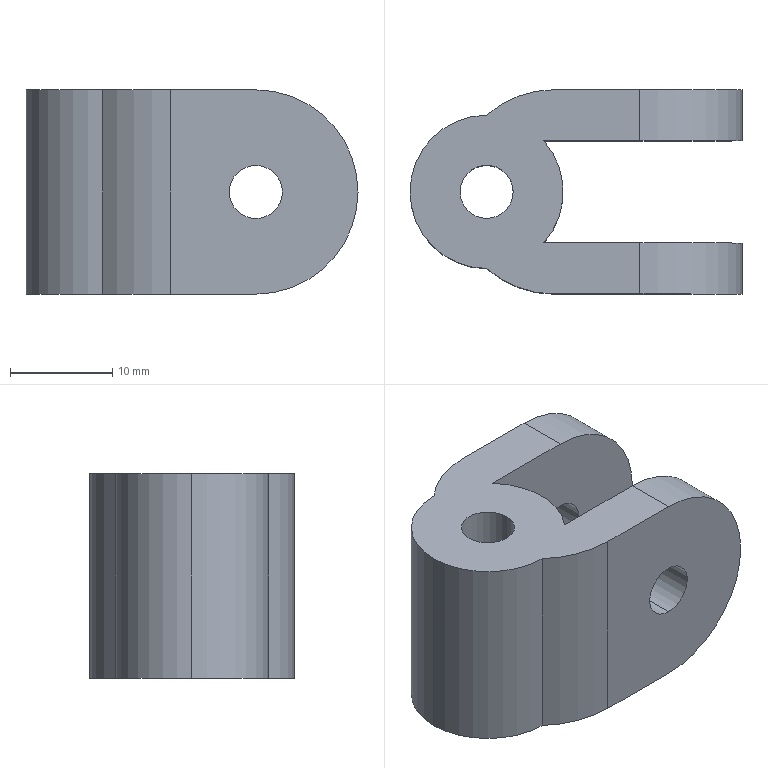Part | SolidWorks | features Fillet 2, ICE 2, Extrusion 1 | 1 solid | 21 faces | box 32.5 x 20 x 20 mm | volume 6873 mm3 | cylinder 15 | plane 6 | commonest cylinder face diameters 5.2 x6 20 x6 15 x3
STEP:
#1=CARTESIAN_POINT('',(15.,10.,2.6));
#2=VERTEX_POINT('',#1);
#3=CARTESIAN_POINT('',(15.,10.,-2.6));
#4=VERTEX_POINT('',#3);
#5=CARTESIAN_POINT('',(15.,10.,0.));
#6=DIRECTION('',(0.,-1.,0.));
#7=DIRECTION('',(0.,0.,-1.));
#8=AXIS2_PLACEMENT_3D('',#5,#6,#7);
#9=CIRCLE('',#8,2.6);
#10=EDGE_CURVE('',#2,#4,#9,.T.);
#11=ORIENTED_EDGE('',*,*,#10,.F.);
#12=CARTESIAN_POINT('',(15.,5.,2.6));
#13=VERTEX_POINT('',#12);
#14=CARTESIAN_POINT('',(15.,10.,2.6));
#15=DIRECTION('',(0.,-1.,0.));
#16=VECTOR('',#15,1000.);
#17=LINE('',#14,#16);
#18=EDGE_CURVE('',#2,#13,#17,.T.);
#19=ORIENTED_EDGE('',*,*,#18,.T.);
#20=CARTESIAN_POINT('',(15.,5.,-2.6));
#21=VERTEX_POINT('',#20);
#22=CARTESIAN_POINT('',(15.,5.,0.));
#23=DIRECTION('',(0.,1.,0.));
#24=DIRECTION('',(0.,0.,1.));
#25=AXIS2_PLACEMENT_3D('',#22,#23,#24);
#26=CIRCLE('',#25,2.6);
#27=EDGE_CURVE('',#21,#13,#26,.T.);
#28=ORIENTED_EDGE('',*,*,#27,.F.);
#29=CARTESIAN_POINT('',(15.,10.,-2.6));
#30=DIRECTION('',(0.,-1.,0.));
#31=VECTOR('',#30,1000.);
#32=LINE('',#29,#31);
#33=EDGE_CURVE('',#4,#21,#32,.T.);
#34=ORIENTED_EDGE('',*,*,#33,.F.);
#35=EDGE_LOOP('',(#11,#19,#28,#34));
#36=FACE_OUTER_BOUND('',#35,.T.);
#37=CARTESIAN_POINT('',(15.,10.,0.));
#38=DIRECTION('',(0.,-1.,0.));
#39=DIRECTION('',(0.,0.,-1.));
#40=AXIS2_PLACEMENT_3D('',#37,#38,#39);
#41=CYLINDRICAL_SURFACE('',#40,2.6);
#42=ADVANCED_FACE('',(#36),#41,.F.);
#43=CARTESIAN_POINT('',(15.,-5.,2.6));
#44=VERTEX_POINT('',#43);
#45=CARTESIAN_POINT('',(15.,-5.,-2.6));
#46=VERTEX_POINT('',#45);
#47=CARTESIAN_POINT('',(15.,-5.,0.));
#48=DIRECTION('',(0.,-1.,0.));
#49=DIRECTION('',(0.,0.,-1.));
#50=AXIS2_PLACEMENT_3D('',#47,#48,#49);
#51=CIRCLE('',#50,2.6);
#52=EDGE_CURVE('',#44,#46,#51,.T.);
#53=ORIENTED_EDGE('',*,*,#52,.F.);
#54=CARTESIAN_POINT('',(15.,-10.,2.6));
#55=VERTEX_POINT('',#54);
#56=CARTESIAN_POINT('',(15.,10.,2.6));
#57=DIRECTION('',(0.,-1.,0.));
#58=VECTOR('',#57,1000.);
#59=LINE('',#56,#58);
#60=EDGE_CURVE('',#44,#55,#59,.T.);
#61=ORIENTED_EDGE('',*,*,#60,.T.);
#62=CARTESIAN_POINT('',(15.,-10.,-2.6));
#63=VERTEX_POINT('',#62);
#64=CARTESIAN_POINT('',(15.,-10.,0.));
#65=DIRECTION('',(0.,-1.,0.));
#66=DIRECTION('',(0.,0.,-1.));
#67=AXIS2_PLACEMENT_3D('',#64,#65,#66);
#68=CIRCLE('',#67,2.6);
#69=EDGE_CURVE('',#55,#63,#68,.T.);
#70=ORIENTED_EDGE('',*,*,#69,.T.);
#71=CARTESIAN_POINT('',(15.,10.,-2.6));
#72=DIRECTION('',(0.,-1.,0.));
#73=VECTOR('',#72,1000.);
#74=LINE('',#71,#73);
#75=EDGE_CURVE('',#46,#63,#74,.T.);
#76=ORIENTED_EDGE('',*,*,#75,.F.);
#77=EDGE_LOOP('',(#53,#61,#70,#76));
#78=FACE_OUTER_BOUND('',#77,.T.);
#79=CARTESIAN_POINT('',(15.,10.,0.));
#80=DIRECTION('',(0.,-1.,0.));
#81=DIRECTION('',(0.,0.,-1.));
#82=AXIS2_PLACEMENT_3D('',#79,#80,#81);
#83=CYLINDRICAL_SURFACE('',#82,2.6);
#84=ADVANCED_FACE('',(#78),#83,.F.);
#85=CARTESIAN_POINT('',(-2.6,0.,10.));
#86=VERTEX_POINT('',#85);
#87=CARTESIAN_POINT('',(2.6,0.,10.));
#88=VERTEX_POINT('',#87);
#89=CARTESIAN_POINT('',(0.,0.,10.));
#90=DIRECTION('',(0.,0.,1.));
#91=DIRECTION('',(1.,0.,0.));
#92=AXIS2_PLACEMENT_3D('',#89,#90,#91);
#93=CIRCLE('',#92,2.6);
#94=EDGE_CURVE('',#86,#88,#93,.T.);
#95=ORIENTED_EDGE('',*,*,#94,.T.);
#96=CARTESIAN_POINT('',(2.6,0.,-10.));
#97=VERTEX_POINT('',#96);
#98=CARTESIAN_POINT('',(2.6,0.,10.));
#99=DIRECTION('',(0.,0.,-1.));
#100=VECTOR('',#99,1000.);
#101=LINE('',#98,#100);
#102=EDGE_CURVE('',#88,#97,#101,.T.);
#103=ORIENTED_EDGE('',*,*,#102,.T.);
#104=CARTESIAN_POINT('',(-2.6,0.,-10.));
#105=VERTEX_POINT('',#104);
#106=CARTESIAN_POINT('',(0.,0.,-10.));
#107=DIRECTION('',(0.,0.,1.));
#108=DIRECTION('',(1.,0.,0.));
#109=AXIS2_PLACEMENT_3D('',#106,#107,#108);
#110=CIRCLE('',#109,2.6);
#111=EDGE_CURVE('',#105,#97,#110,.T.);
#112=ORIENTED_EDGE('',*,*,#111,.F.);
#113=CARTESIAN_POINT('',(-2.6,0.,10.));
#114=DIRECTION('',(0.,0.,-1.));
#115=VECTOR('',#114,1000.);
#116=LINE('',#113,#115);
#117=EDGE_CURVE('',#86,#105,#116,.T.);
#118=ORIENTED_EDGE('',*,*,#117,.F.);
#119=EDGE_LOOP('',(#95,#103,#112,#118));
#120=FACE_OUTER_BOUND('',#119,.T.);
#121=CARTESIAN_POINT('',(0.,0.,10.));
#122=DIRECTION('',(0.,0.,-1.));
#123=DIRECTION('',(-1.,0.,0.));
#124=AXIS2_PLACEMENT_3D('',#121,#122,#123);
#125=CYLINDRICAL_SURFACE('',#124,2.6);
#126=ADVANCED_FACE('',(#120),#125,.F.);
#127=CARTESIAN_POINT('',(-7.5,0.,10.));
#128=VERTEX_POINT('',#127);
#129=CARTESIAN_POINT('',(0.,-7.5,10.));
#130=VERTEX_POINT('',#129);
#131=CARTESIAN_POINT('',(0.,0.,10.));
#132=DIRECTION('',(0.,0.,1.));
#133=DIRECTION('',(1.,0.,0.));
#134=AXIS2_PLACEMENT_3D('',#131,#132,#133);
#135=CIRCLE('',#134,7.5);
#136=EDGE_CURVE('',#128,#130,#135,.T.);
#137=ORIENTED_EDGE('',*,*,#136,.F.);
#138=CARTESIAN_POINT('',(-7.5,0.,-10.));
#139=VERTEX_POINT('',#138);
#140=CARTESIAN_POINT('',(-7.5,0.,10.));
#141=DIRECTION('',(0.,0.,-1.));
#142=VECTOR('',#141,1000.);
#143=LINE('',#140,#142);
#144=EDGE_CURVE('',#128,#139,#143,.T.);
#145=ORIENTED_EDGE('',*,*,#144,.T.);
#146=CARTESIAN_POINT('',(0.,-7.5,-10.));
#147=VERTEX_POINT('',#146);
#148=CARTESIAN_POINT('',(0.,0.,-10.));
#149=DIRECTION('',(0.,0.,1.));
#150=DIRECTION('',(1.,0.,0.));
#151=AXIS2_PLACEMENT_3D('',#148,#149,#150);
#152=CIRCLE('',#151,7.5);
#153=EDGE_CURVE('',#139,#147,#152,.T.);
#154=ORIENTED_EDGE('',*,*,#153,.T.);
#155=CARTESIAN_POINT('',(0.,-7.5,10.));
#156=DIRECTION('',(0.,0.,-1.));
#157=VECTOR('',#156,1000.);
#158=LINE('',#155,#157);
#159=EDGE_CURVE('',#130,#147,#158,.T.);
#160=ORIENTED_EDGE('',*,*,#159,.F.);
#161=EDGE_LOOP('',(#137,#145,#154,#160));
#162=FACE_OUTER_BOUND('',#161,.T.);
#163=CARTESIAN_POINT('',(0.,0.,10.));
#164=DIRECTION('',(0.,0.,-1.));
#165=DIRECTION('',(-1.,0.,0.));
#166=AXIS2_PLACEMENT_3D('',#163,#164,#165);
#167=CYLINDRICAL_SURFACE('',#166,7.5);
#168=ADVANCED_FACE('',(#162),#167,.T.);
#169=CARTESIAN_POINT('',(5.59,-5.,-10.));
#170=VERTEX_POINT('',#169);
#171=CARTESIAN_POINT('',(5.59,-5.,10.));
#172=VERTEX_POINT('',#171);
#173=CARTESIAN_POINT('',(5.59,-5.,10.));
#174=DIRECTION('',(0.,0.,1.));
#175=VECTOR('',#174,1000.);
#176=LINE('',#173,#175);
#177=EDGE_CURVE('',#170,#172,#176,.T.);
#178=ORIENTED_EDGE('',*,*,#177,.F.);
#179=CARTESIAN_POINT('',(5.59,5.,-10.));
#180=VERTEX_POINT('',#179);
#181=CARTESIAN_POINT('',(0.,0.,-10.));
#182=DIRECTION('',(0.,0.,1.));
#183=DIRECTION('',(1.,0.,0.));
#184=AXIS2_PLACEMENT_3D('',#181,#182,#183);
#185=CIRCLE('',#184,7.5);
#186=EDGE_CURVE('',#170,#180,#185,.T.);
#187=ORIENTED_EDGE('',*,*,#186,.T.);
#188=CARTESIAN_POINT('',(5.59,5.,10.));
#189=VERTEX_POINT('',#188);
#190=CARTESIAN_POINT('',(5.59,5.,10.));
#191=DIRECTION('',(0.,0.,-1.));
#192=VECTOR('',#191,1000.);
#193=LINE('',#190,#192);
#194=EDGE_CURVE('',#189,#180,#193,.T.);
#195=ORIENTED_EDGE('',*,*,#194,.F.);
#196=CARTESIAN_POINT('',(0.,0.,10.));
#197=DIRECTION('',(0.,0.,1.));
#198=DIRECTION('',(1.,0.,0.));
#199=AXIS2_PLACEMENT_3D('',#196,#197,#198);
#200=CIRCLE('',#199,7.5);
#201=EDGE_CURVE('',#172,#189,#200,.T.);
#202=ORIENTED_EDGE('',*,*,#201,.F.);
#203=EDGE_LOOP('',(#178,#187,#195,#202));
#204=FACE_OUTER_BOUND('',#203,.T.);
#205=CARTESIAN_POINT('',(0.,0.,10.));
#206=DIRECTION('',(0.,0.,-1.));
#207=DIRECTION('',(-1.,0.,0.));
#208=AXIS2_PLACEMENT_3D('',#205,#206,#207);
#209=CYLINDRICAL_SURFACE('',#208,7.5);
#210=ADVANCED_FACE('',(#204),#209,.T.);
#211=ORIENTED_EDGE('',*,*,#144,.F.);
#212=CARTESIAN_POINT('',(0.,7.5,10.));
#213=VERTEX_POINT('',#212);
#214=CARTESIAN_POINT('',(0.,0.,10.));
#215=DIRECTION('',(0.,0.,1.));
#216=DIRECTION('',(1.,0.,0.));
#217=AXIS2_PLACEMENT_3D('',#214,#215,#216);
#218=CIRCLE('',#217,7.5);
#219=EDGE_CURVE('',#213,#128,#218,.T.);
#220=ORIENTED_EDGE('',*,*,#219,.F.);
#221=CARTESIAN_POINT('',(0.,7.5,-10.));
#222=VERTEX_POINT('',#221);
#223=CARTESIAN_POINT('',(0.,7.5,10.));
#224=DIRECTION('',(0.,0.,1.));
#225=VECTOR('',#224,1000.);
#226=LINE('',#223,#225);
#227=EDGE_CURVE('',#222,#213,#226,.T.);
#228=ORIENTED_EDGE('',*,*,#227,.F.);
#229=CARTESIAN_POINT('',(0.,0.,-10.));
#230=DIRECTION('',(0.,0.,1.));
#231=DIRECTION('',(1.,0.,0.));
#232=AXIS2_PLACEMENT_3D('',#229,#230,#231);
#233=CIRCLE('',#232,7.5);
#234=EDGE_CURVE('',#222,#139,#233,.T.);
#235=ORIENTED_EDGE('',*,*,#234,.T.);
#236=EDGE_LOOP('',(#211,#220,#228,#235));
#237=FACE_OUTER_BOUND('',#236,.T.);
#238=CARTESIAN_POINT('',(0.,0.,10.));
#239=DIRECTION('',(0.,0.,-1.));
#240=DIRECTION('',(-1.,0.,0.));
#241=AXIS2_PLACEMENT_3D('',#238,#239,#240);
#242=CYLINDRICAL_SURFACE('',#241,7.5);
#243=ADVANCED_FACE('',(#237),#242,.T.);
#244=CARTESIAN_POINT('',(15.,5.,10.));
#245=VERTEX_POINT('',#244);
#246=CARTESIAN_POINT('',(0.,5.,10.));
#247=DIRECTION('',(1.,0.,0.));
#248=VECTOR('',#247,1000.);
#249=LINE('',#246,#248);
#250=EDGE_CURVE('',#189,#245,#249,.T.);
#251=ORIENTED_EDGE('',*,*,#250,.T.);
#252=CARTESIAN_POINT('',(15.,10.,10.));
#253=VERTEX_POINT('',#252);
#254=CARTESIAN_POINT('',(15.,10.,10.));
#255=DIRECTION('',(0.,1.,0.));
#256=VECTOR('',#255,1000.);
#257=LINE('',#254,#256);
#258=EDGE_CURVE('',#245,#253,#257,.T.);
#259=ORIENTED_EDGE('',*,*,#258,.T.);
#260=CARTESIAN_POINT('',(6.614,10.,10.));
#261=VERTEX_POINT('',#260);
#262=CARTESIAN_POINT('',(0.,10.,10.));
#263=DIRECTION('',(-1.,0.,0.));
#264=VECTOR('',#263,1000.);
#265=LINE('',#262,#264);
#266=EDGE_CURVE('',#253,#261,#265,.T.);
#267=ORIENTED_EDGE('',*,*,#266,.T.);
#268=CARTESIAN_POINT('',(6.614,0.,10.));
#269=DIRECTION('',(0.,0.,1.));
#270=DIRECTION('',(1.,0.,0.));
#271=AXIS2_PLACEMENT_3D('',#268,#269,#270);
#272=CIRCLE('',#271,10.);
#273=EDGE_CURVE('',#261,#213,#272,.T.);
#274=ORIENTED_EDGE('',*,*,#273,.T.);
#275=ORIENTED_EDGE('',*,*,#219,.T.);
#276=ORIENTED_EDGE('',*,*,#136,.T.);
#277=CARTESIAN_POINT('',(6.614,-10.,10.));
#278=VERTEX_POINT('',#277);
#279=CARTESIAN_POINT('',(6.614,0.,10.));
#280=DIRECTION('',(0.,0.,1.));
#281=DIRECTION('',(1.,0.,0.));
#282=AXIS2_PLACEMENT_3D('',#279,#280,#281);
#283=CIRCLE('',#282,10.);
#284=EDGE_CURVE('',#130,#278,#283,.T.);
#285=ORIENTED_EDGE('',*,*,#284,.T.);
#286=CARTESIAN_POINT('',(15.,-10.,10.));
#287=VERTEX_POINT('',#286);
#288=CARTESIAN_POINT('',(0.,-10.,10.));
#289=DIRECTION('',(1.,0.,0.));
#290=VECTOR('',#289,1000.);
#291=LINE('',#288,#290);
#292=EDGE_CURVE('',#278,#287,#291,.T.);
#293=ORIENTED_EDGE('',*,*,#292,.T.);
#294=CARTESIAN_POINT('',(15.,-5.,10.));
#295=VERTEX_POINT('',#294);
#296=CARTESIAN_POINT('',(15.,-5.,10.));
#297=DIRECTION('',(0.,1.,0.));
#298=VECTOR('',#297,1000.);
#299=LINE('',#296,#298);
#300=EDGE_CURVE('',#287,#295,#299,.T.);
#301=ORIENTED_EDGE('',*,*,#300,.T.);
#302=CARTESIAN_POINT('',(0.,-5.,10.));
#303=DIRECTION('',(-1.,0.,0.));
#304=VECTOR('',#303,1000.);
#305=LINE('',#302,#304);
#306=EDGE_CURVE('',#295,#172,#305,.T.);
#307=ORIENTED_EDGE('',*,*,#306,.T.);
#308=ORIENTED_EDGE('',*,*,#201,.T.);
#309=EDGE_LOOP('',(#251,#259,#267,#274,#275,#276,#285,#293,#301,#307,#308));
#310=FACE_OUTER_BOUND('',#309,.T.);
#311=ORIENTED_EDGE('',*,*,#94,.F.);
#312=CARTESIAN_POINT('',(0.,0.,10.));
#313=DIRECTION('',(0.,0.,1.));
#314=DIRECTION('',(1.,0.,0.));
#315=AXIS2_PLACEMENT_3D('',#312,#313,#314);
#316=CIRCLE('',#315,2.6);
#317=EDGE_CURVE('',#88,#86,#316,.T.);
#318=ORIENTED_EDGE('',*,*,#317,.F.);
#319=EDGE_LOOP('',(#311,#318));
#320=FACE_BOUND('',#319,.T.);
#321=CARTESIAN_POINT('',(0.,0.,10.));
#322=DIRECTION('',(0.,0.,1.));
#323=DIRECTION('',(1.,0.,0.));
#324=AXIS2_PLACEMENT_3D('',#321,#322,#323);
#325=PLANE('',#324);
#326=ADVANCED_FACE('',(#310,#320),#325,.T.);
#327=CARTESIAN_POINT('',(15.,-5.,-10.));
#328=VERTEX_POINT('',#327);
#329=CARTESIAN_POINT('',(0.,-5.,-10.));
#330=DIRECTION('',(-1.,0.,0.));
#331=VECTOR('',#330,1000.);
#332=LINE('',#329,#331);
#333=EDGE_CURVE('',#328,#170,#332,.T.);
#334=ORIENTED_EDGE('',*,*,#333,.F.);
#335=CARTESIAN_POINT('',(15.,-10.,-10.));
#336=VERTEX_POINT('',#335);
#337=CARTESIAN_POINT('',(15.,0.,-10.));
#338=DIRECTION('',(0.,-1.,0.));
#339=VECTOR('',#338,1000.);
#340=LINE('',#337,#339);
#341=EDGE_CURVE('',#328,#336,#340,.T.);
#342=ORIENTED_EDGE('',*,*,#341,.T.);
#343=CARTESIAN_POINT('',(6.614,-10.,-10.));
#344=VERTEX_POINT('',#343);
#345=CARTESIAN_POINT('',(0.,-10.,-10.));
#346=DIRECTION('',(1.,0.,0.));
#347=VECTOR('',#346,1000.);
#348=LINE('',#345,#347);
#349=EDGE_CURVE('',#344,#336,#348,.T.);
#350=ORIENTED_EDGE('',*,*,#349,.F.);
#351=CARTESIAN_POINT('',(6.614,0.,-10.));
#352=DIRECTION('',(0.,0.,-1.));
#353=DIRECTION('',(1.,0.,0.));
#354=AXIS2_PLACEMENT_3D('',#351,#352,#353);
#355=CIRCLE('',#354,10.);
#356=EDGE_CURVE('',#344,#147,#355,.T.);
#357=ORIENTED_EDGE('',*,*,#356,.T.);
#358=ORIENTED_EDGE('',*,*,#153,.F.);
#359=ORIENTED_EDGE('',*,*,#234,.F.);
#360=CARTESIAN_POINT('',(6.614,10.,-10.));
#361=VERTEX_POINT('',#360);
#362=CARTESIAN_POINT('',(6.614,0.,-10.));
#363=DIRECTION('',(0.,0.,-1.));
#364=DIRECTION('',(1.,0.,0.));
#365=AXIS2_PLACEMENT_3D('',#362,#363,#364);
#366=CIRCLE('',#365,10.);
#367=EDGE_CURVE('',#222,#361,#366,.T.);
#368=ORIENTED_EDGE('',*,*,#367,.T.);
#369=CARTESIAN_POINT('',(15.,10.,-10.));
#370=VERTEX_POINT('',#369);
#371=CARTESIAN_POINT('',(0.,10.,-10.));
#372=DIRECTION('',(-1.,0.,0.));
#373=VECTOR('',#372,1000.);
#374=LINE('',#371,#373);
#375=EDGE_CURVE('',#370,#361,#374,.T.);
#376=ORIENTED_EDGE('',*,*,#375,.F.);
#377=CARTESIAN_POINT('',(15.,5.,-10.));
#378=VERTEX_POINT('',#377);
#379=CARTESIAN_POINT('',(15.,0.,-10.));
#380=DIRECTION('',(0.,-1.,0.));
#381=VECTOR('',#380,1000.);
#382=LINE('',#379,#381);
#383=EDGE_CURVE('',#370,#378,#382,.T.);
#384=ORIENTED_EDGE('',*,*,#383,.T.);
#385=CARTESIAN_POINT('',(0.,5.,-10.));
#386=DIRECTION('',(1.,0.,0.));
#387=VECTOR('',#386,1000.);
#388=LINE('',#385,#387);
#389=EDGE_CURVE('',#180,#378,#388,.T.);
#390=ORIENTED_EDGE('',*,*,#389,.F.);
#391=ORIENTED_EDGE('',*,*,#186,.F.);
#392=EDGE_LOOP('',(#334,#342,#350,#357,#358,#359,#368,#376,#384,#390,#391));
#393=FACE_OUTER_BOUND('',#392,.T.);
#394=ORIENTED_EDGE('',*,*,#111,.T.);
#395=CARTESIAN_POINT('',(0.,0.,-10.));
#396=DIRECTION('',(0.,0.,1.));
#397=DIRECTION('',(1.,0.,0.));
#398=AXIS2_PLACEMENT_3D('',#395,#396,#397);
#399=CIRCLE('',#398,2.6);
#400=EDGE_CURVE('',#97,#105,#399,.T.);
#401=ORIENTED_EDGE('',*,*,#400,.T.);
#402=EDGE_LOOP('',(#394,#401));
#403=FACE_BOUND('',#402,.T.);
#404=CARTESIAN_POINT('',(0.,0.,-10.));
#405=DIRECTION('',(0.,0.,1.));
#406=DIRECTION('',(1.,0.,0.));
#407=AXIS2_PLACEMENT_3D('',#404,#405,#406);
#408=PLANE('',#407);
#409=ADVANCED_FACE('',(#393,#403),#408,.F.);
#410=ORIENTED_EDGE('',*,*,#102,.F.);
#411=ORIENTED_EDGE('',*,*,#317,.T.);
#412=ORIENTED_EDGE('',*,*,#117,.T.);
#413=ORIENTED_EDGE('',*,*,#400,.F.);
#414=EDGE_LOOP('',(#410,#411,#412,#413));
#415=FACE_OUTER_BOUND('',#414,.T.);
#416=CARTESIAN_POINT('',(0.,0.,10.));
#417=DIRECTION('',(0.,0.,-1.));
#418=DIRECTION('',(-1.,0.,0.));
#419=AXIS2_PLACEMENT_3D('',#416,#417,#418);
#420=CYLINDRICAL_SURFACE('',#419,2.6);
#421=ADVANCED_FACE('',(#415),#420,.F.);
#422=ORIENTED_EDGE('',*,*,#27,.T.);
#423=CARTESIAN_POINT('',(15.,5.,0.));
#424=DIRECTION('',(0.,1.,0.));
#425=DIRECTION('',(0.,0.,1.));
#426=AXIS2_PLACEMENT_3D('',#423,#424,#425);
#427=CIRCLE('',#426,2.6);
#428=EDGE_CURVE('',#13,#21,#427,.T.);
#429=ORIENTED_EDGE('',*,*,#428,.T.);
#430=EDGE_LOOP('',(#422,#429));
#431=FACE_BOUND('',#430,.T.);
#432=ORIENTED_EDGE('',*,*,#389,.T.);
#433=CARTESIAN_POINT('',(25.,5.,0.));
#434=VERTEX_POINT('',#433);
#435=CARTESIAN_POINT('',(15.,5.,0.));
#436=DIRECTION('',(0.,-1.,0.));
#437=DIRECTION('',(0.,0.,1.));
#438=AXIS2_PLACEMENT_3D('',#435,#436,#437);
#439=CIRCLE('',#438,10.);
#440=EDGE_CURVE('',#378,#434,#439,.T.);
#441=ORIENTED_EDGE('',*,*,#440,.T.);
#442=CARTESIAN_POINT('',(15.,5.,0.));
#443=DIRECTION('',(0.,-1.,0.));
#444=DIRECTION('',(0.,0.,1.));
#445=AXIS2_PLACEMENT_3D('',#442,#443,#444);
#446=CIRCLE('',#445,10.);
#447=EDGE_CURVE('',#434,#245,#446,.T.);
#448=ORIENTED_EDGE('',*,*,#447,.T.);
#449=ORIENTED_EDGE('',*,*,#250,.F.);
#450=ORIENTED_EDGE('',*,*,#194,.T.);
#451=EDGE_LOOP('',(#432,#441,#448,#449,#450));
#452=FACE_OUTER_BOUND('',#451,.T.);
#453=CARTESIAN_POINT('',(0.,5.,10.));
#454=DIRECTION('',(0.,1.,0.));
#455=DIRECTION('',(0.,0.,1.));
#456=AXIS2_PLACEMENT_3D('',#453,#454,#455);
#457=PLANE('',#456);
#458=ADVANCED_FACE('',(#431,#452),#457,.F.);
#459=CARTESIAN_POINT('',(15.,10.,0.));
#460=DIRECTION('',(0.,-1.,0.));
#461=DIRECTION('',(0.,0.,-1.));
#462=AXIS2_PLACEMENT_3D('',#459,#460,#461);
#463=CIRCLE('',#462,2.6);
#464=EDGE_CURVE('',#4,#2,#463,.T.);
#465=ORIENTED_EDGE('',*,*,#464,.T.);
#466=ORIENTED_EDGE('',*,*,#10,.T.);
#467=EDGE_LOOP('',(#465,#466));
#468=FACE_BOUND('',#467,.T.);
#469=CARTESIAN_POINT('',(25.,10.,0.));
#470=VERTEX_POINT('',#469);
#471=CARTESIAN_POINT('',(15.,10.,0.));
#472=DIRECTION('',(0.,1.,0.));
#473=DIRECTION('',(0.,0.,-1.));
#474=AXIS2_PLACEMENT_3D('',#471,#472,#473);
#475=CIRCLE('',#474,10.);
#476=EDGE_CURVE('',#253,#470,#475,.T.);
#477=ORIENTED_EDGE('',*,*,#476,.T.);
#478=CARTESIAN_POINT('',(15.,10.,0.));
#479=DIRECTION('',(0.,1.,0.));
#480=DIRECTION('',(0.,0.,-1.));
#481=AXIS2_PLACEMENT_3D('',#478,#479,#480);
#482=CIRCLE('',#481,10.);
#483=EDGE_CURVE('',#470,#370,#482,.T.);
#484=ORIENTED_EDGE('',*,*,#483,.T.);
#485=ORIENTED_EDGE('',*,*,#375,.T.);
#486=CARTESIAN_POINT('',(6.614,10.,10.));
#487=DIRECTION('',(0.,0.,1.));
#488=VECTOR('',#487,1000.);
#489=LINE('',#486,#488);
#490=EDGE_CURVE('',#361,#261,#489,.T.);
#491=ORIENTED_EDGE('',*,*,#490,.T.);
#492=ORIENTED_EDGE('',*,*,#266,.F.);
#493=EDGE_LOOP('',(#477,#484,#485,#491,#492));
#494=FACE_OUTER_BOUND('',#493,.T.);
#495=CARTESIAN_POINT('',(0.,10.,10.));
#496=DIRECTION('',(0.,-1.,0.));
#497=DIRECTION('',(0.,0.,-1.));
#498=AXIS2_PLACEMENT_3D('',#495,#496,#497);
#499=PLANE('',#498);
#500=ADVANCED_FACE('',(#468,#494),#499,.F.);
#501=CARTESIAN_POINT('',(15.,-5.,0.));
#502=DIRECTION('',(0.,-1.,0.));
#503=DIRECTION('',(0.,0.,-1.));
#504=AXIS2_PLACEMENT_3D('',#501,#502,#503);
#505=CIRCLE('',#504,2.6);
#506=EDGE_CURVE('',#46,#44,#505,.T.);
#507=ORIENTED_EDGE('',*,*,#506,.T.);
#508=ORIENTED_EDGE('',*,*,#52,.T.);
#509=EDGE_LOOP('',(#507,#508));
#510=FACE_BOUND('',#509,.T.);
#511=CARTESIAN_POINT('',(25.,-5.,0.));
#512=VERTEX_POINT('',#511);
#513=CARTESIAN_POINT('',(15.,-5.,0.));
#514=DIRECTION('',(0.,1.,0.));
#515=DIRECTION('',(0.,0.,-1.));
#516=AXIS2_PLACEMENT_3D('',#513,#514,#515);
#517=CIRCLE('',#516,10.);
#518=EDGE_CURVE('',#295,#512,#517,.T.);
#519=ORIENTED_EDGE('',*,*,#518,.T.);
#520=CARTESIAN_POINT('',(15.,-5.,0.));
#521=DIRECTION('',(0.,1.,0.));
#522=DIRECTION('',(0.,0.,-1.));
#523=AXIS2_PLACEMENT_3D('',#520,#521,#522);
#524=CIRCLE('',#523,10.);
#525=EDGE_CURVE('',#512,#328,#524,.T.);
#526=ORIENTED_EDGE('',*,*,#525,.T.);
#527=ORIENTED_EDGE('',*,*,#333,.T.);
#528=ORIENTED_EDGE('',*,*,#177,.T.);
#529=ORIENTED_EDGE('',*,*,#306,.F.);
#530=EDGE_LOOP('',(#519,#526,#527,#528,#529));
#531=FACE_OUTER_BOUND('',#530,.T.);
#532=CARTESIAN_POINT('',(0.,-5.,10.));
#533=DIRECTION('',(0.,-1.,0.));
#534=DIRECTION('',(0.,0.,-1.));
#535=AXIS2_PLACEMENT_3D('',#532,#533,#534);
#536=PLANE('',#535);
#537=ADVANCED_FACE('',(#510,#531),#536,.F.);
#538=CARTESIAN_POINT('',(15.,-10.,0.));
#539=DIRECTION('',(0.,-1.,0.));
#540=DIRECTION('',(0.,0.,-1.));
#541=AXIS2_PLACEMENT_3D('',#538,#539,#540);
#542=CIRCLE('',#541,2.6);
#543=EDGE_CURVE('',#63,#55,#542,.T.);
#544=ORIENTED_EDGE('',*,*,#543,.F.);
#545=ORIENTED_EDGE('',*,*,#69,.F.);
#546=EDGE_LOOP('',(#544,#545));
#547=FACE_BOUND('',#546,.T.);
#548=ORIENTED_EDGE('',*,*,#349,.T.);
#549=CARTESIAN_POINT('',(25.,-10.,0.));
#550=VERTEX_POINT('',#549);
#551=CARTESIAN_POINT('',(15.,-10.,0.));
#552=DIRECTION('',(0.,-1.,0.));
#553=DIRECTION('',(0.,0.,1.));
#554=AXIS2_PLACEMENT_3D('',#551,#552,#553);
#555=CIRCLE('',#554,10.);
#556=EDGE_CURVE('',#336,#550,#555,.T.);
#557=ORIENTED_EDGE('',*,*,#556,.T.);
#558=CARTESIAN_POINT('',(15.,-10.,0.));
#559=DIRECTION('',(0.,-1.,0.));
#560=DIRECTION('',(0.,0.,1.));
#561=AXIS2_PLACEMENT_3D('',#558,#559,#560);
#562=CIRCLE('',#561,10.);
#563=EDGE_CURVE('',#550,#287,#562,.T.);
#564=ORIENTED_EDGE('',*,*,#563,.T.);
#565=ORIENTED_EDGE('',*,*,#292,.F.);
#566=CARTESIAN_POINT('',(6.614,-10.,10.));
#567=DIRECTION('',(0.,0.,-1.));
#568=VECTOR('',#567,1000.);
#569=LINE('',#566,#568);
#570=EDGE_CURVE('',#278,#344,#569,.T.);
#571=ORIENTED_EDGE('',*,*,#570,.T.);
#572=EDGE_LOOP('',(#548,#557,#564,#565,#571));
#573=FACE_OUTER_BOUND('',#572,.T.);
#574=CARTESIAN_POINT('',(0.,-10.,10.));
#575=DIRECTION('',(0.,1.,0.));
#576=DIRECTION('',(0.,0.,1.));
#577=AXIS2_PLACEMENT_3D('',#574,#575,#576);
#578=PLANE('',#577);
#579=ADVANCED_FACE('',(#547,#573),#578,.F.);
#580=ORIENTED_EDGE('',*,*,#284,.F.);
#581=ORIENTED_EDGE('',*,*,#159,.T.);
#582=ORIENTED_EDGE('',*,*,#356,.F.);
#583=ORIENTED_EDGE('',*,*,#570,.F.);
#584=EDGE_LOOP('',(#580,#581,#582,#583));
#585=FACE_OUTER_BOUND('',#584,.T.);
#586=CARTESIAN_POINT('',(6.614,0.,10.));
#587=DIRECTION('',(0.,0.,-1.));
#588=DIRECTION('',(-1.,0.,0.));
#589=AXIS2_PLACEMENT_3D('',#586,#587,#588);
#590=CYLINDRICAL_SURFACE('',#589,10.);
#591=ADVANCED_FACE('',(#585),#590,.T.);
#592=ORIENTED_EDGE('',*,*,#273,.F.);
#593=ORIENTED_EDGE('',*,*,#490,.F.);
#594=ORIENTED_EDGE('',*,*,#367,.F.);
#595=ORIENTED_EDGE('',*,*,#227,.T.);
#596=EDGE_LOOP('',(#592,#593,#594,#595));
#597=FACE_OUTER_BOUND('',#596,.T.);
#598=CARTESIAN_POINT('',(6.614,0.,10.));
#599=DIRECTION('',(0.,0.,-1.));
#600=DIRECTION('',(-1.,0.,0.));
#601=AXIS2_PLACEMENT_3D('',#598,#599,#600);
#602=CYLINDRICAL_SURFACE('',#601,10.);
#603=ADVANCED_FACE('',(#597),#602,.T.);
#604=ORIENTED_EDGE('',*,*,#300,.F.);
#605=ORIENTED_EDGE('',*,*,#563,.F.);
#606=CARTESIAN_POINT('',(25.,-10.,0.));
#607=DIRECTION('',(0.,-1.,0.));
#608=VECTOR('',#607,1000.);
#609=LINE('',#606,#608);
#610=EDGE_CURVE('',#512,#550,#609,.T.);
#611=ORIENTED_EDGE('',*,*,#610,.F.);
#612=ORIENTED_EDGE('',*,*,#518,.F.);
#613=EDGE_LOOP('',(#604,#605,#611,#612));
#614=FACE_OUTER_BOUND('',#613,.T.);
#615=CARTESIAN_POINT('',(15.,0.,0.));
#616=DIRECTION('',(0.,-1.,0.));
#617=DIRECTION('',(0.,0.,-1.));
#618=AXIS2_PLACEMENT_3D('',#615,#616,#617);
#619=CYLINDRICAL_SURFACE('',#618,10.);
#620=ADVANCED_FACE('',(#614),#619,.T.);
#621=ORIENTED_EDGE('',*,*,#556,.F.);
#622=ORIENTED_EDGE('',*,*,#341,.F.);
#623=ORIENTED_EDGE('',*,*,#525,.F.);
#624=ORIENTED_EDGE('',*,*,#610,.T.);
#625=EDGE_LOOP('',(#621,#622,#623,#624));
#626=FACE_OUTER_BOUND('',#625,.T.);
#627=CARTESIAN_POINT('',(15.,-10.,0.));
#628=DIRECTION('',(0.,1.,0.));
#629=DIRECTION('',(0.,0.,1.));
#630=AXIS2_PLACEMENT_3D('',#627,#628,#629);
#631=CYLINDRICAL_SURFACE('',#630,10.);
#632=ADVANCED_FACE('',(#626),#631,.T.);
#633=ORIENTED_EDGE('',*,*,#258,.F.);
#634=ORIENTED_EDGE('',*,*,#447,.F.);
#635=CARTESIAN_POINT('',(25.,5.,0.));
#636=DIRECTION('',(0.,-1.,0.));
#637=VECTOR('',#636,1000.);
#638=LINE('',#635,#637);
#639=EDGE_CURVE('',#470,#434,#638,.T.);
#640=ORIENTED_EDGE('',*,*,#639,.F.);
#641=ORIENTED_EDGE('',*,*,#476,.F.);
#642=EDGE_LOOP('',(#633,#634,#640,#641));
#643=FACE_OUTER_BOUND('',#642,.T.);
#644=CARTESIAN_POINT('',(15.,0.,0.));
#645=DIRECTION('',(0.,-1.,0.));
#646=DIRECTION('',(0.,0.,-1.));
#647=AXIS2_PLACEMENT_3D('',#644,#645,#646);
#648=CYLINDRICAL_SURFACE('',#647,10.);
#649=ADVANCED_FACE('',(#643),#648,.T.);
#650=ORIENTED_EDGE('',*,*,#440,.F.);
#651=ORIENTED_EDGE('',*,*,#383,.F.);
#652=ORIENTED_EDGE('',*,*,#483,.F.);
#653=ORIENTED_EDGE('',*,*,#639,.T.);
#654=EDGE_LOOP('',(#650,#651,#652,#653));
#655=FACE_OUTER_BOUND('',#654,.T.);
#656=CARTESIAN_POINT('',(15.,10.,0.));
#657=DIRECTION('',(0.,1.,0.));
#658=DIRECTION('',(0.,0.,1.));
#659=AXIS2_PLACEMENT_3D('',#656,#657,#658);
#660=CYLINDRICAL_SURFACE('',#659,10.);
#661=ADVANCED_FACE('',(#655),#660,.T.);
#662=ORIENTED_EDGE('',*,*,#60,.F.);
#663=ORIENTED_EDGE('',*,*,#506,.F.);
#664=ORIENTED_EDGE('',*,*,#75,.T.);
#665=ORIENTED_EDGE('',*,*,#543,.T.);
#666=EDGE_LOOP('',(#662,#663,#664,#665));
#667=FACE_OUTER_BOUND('',#666,.T.);
#668=CARTESIAN_POINT('',(15.,10.,0.));
#669=DIRECTION('',(0.,-1.,0.));
#670=DIRECTION('',(0.,0.,-1.));
#671=AXIS2_PLACEMENT_3D('',#668,#669,#670);
#672=CYLINDRICAL_SURFACE('',#671,2.6);
#673=ADVANCED_FACE('',(#667),#672,.F.);
#674=ORIENTED_EDGE('',*,*,#18,.F.);
#675=ORIENTED_EDGE('',*,*,#464,.F.);
#676=ORIENTED_EDGE('',*,*,#33,.T.);
#677=ORIENTED_EDGE('',*,*,#428,.F.);
#678=EDGE_LOOP('',(#674,#675,#676,#677));
#679=FACE_OUTER_BOUND('',#678,.T.);
#680=CARTESIAN_POINT('',(15.,10.,0.));
#681=DIRECTION('',(0.,-1.,0.));
#682=DIRECTION('',(0.,0.,-1.));
#683=AXIS2_PLACEMENT_3D('',#680,#681,#682);
#684=CYLINDRICAL_SURFACE('',#683,2.6);
#685=ADVANCED_FACE('',(#679),#684,.F.);
#686=CLOSED_SHELL('',(#42,#84,#126,#168,#210,#243,#326,#409,#421,#458,#500,#537,#579,#591,#603,#620,#632,#649,#661,#673,#685));
#687=MANIFOLD_SOLID_BREP('',#686);
#688=CARTESIAN_POINT('',(0.,0.,0.));
#689=DIRECTION('',(0.,0.,1.));
#690=DIRECTION('',(1.,0.,0.));
#691=AXIS2_PLACEMENT_3D('',#688,#689,#690);
#692=(LENGTH_UNIT()NAMED_UNIT(*)SI_UNIT(.MILLI.,.METRE.));
#693=UNCERTAINTY_MEASURE_WITH_UNIT(LENGTH_MEASURE(0.00001),#692,'','');
#694=(NAMED_UNIT(*)PLANE_ANGLE_UNIT()SI_UNIT($,.RADIAN.));
#695=(NAMED_UNIT(*)SI_UNIT($,.STERADIAN.)SOLID_ANGLE_UNIT());
#696=(GEOMETRIC_REPRESENTATION_CONTEXT(3)GLOBAL_UNCERTAINTY_ASSIGNED_CONTEXT((#693))GLOBAL_UNIT_ASSIGNED_CONTEXT((#692,#694,#695))REPRESENTATION_CONTEXT('',''));
#697=ADVANCED_BREP_SHAPE_REPRESENTATION('',(#687,#691),#696);